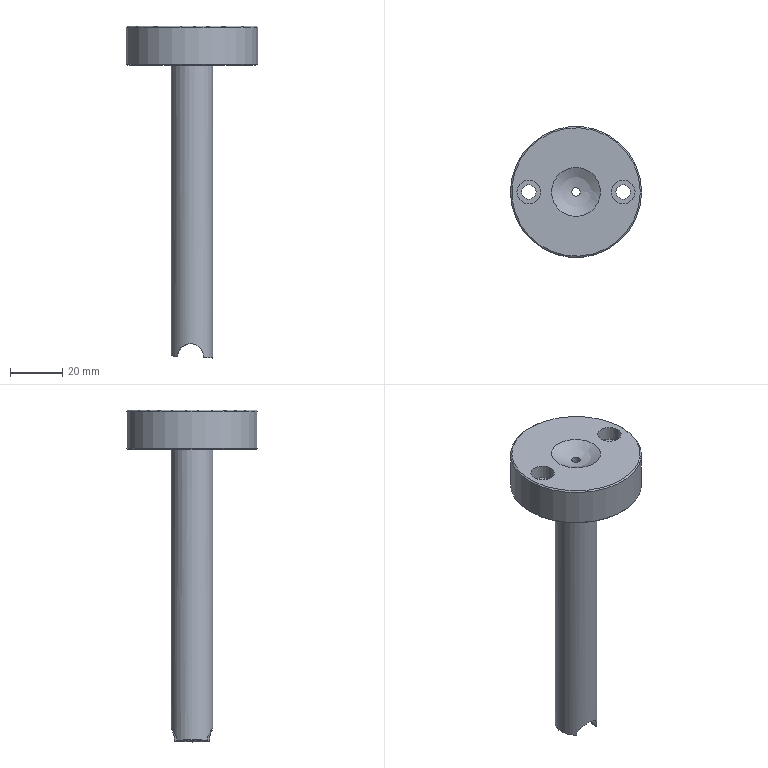Part | STEP file | solid 70 | 1 solid | 18 faces | box 50 x 50 x 126.59 mm | volume 43953 mm3 | cylinder 8 | plane 6 | cone 3 | sphere 1 | commonest cylinder face diameters 5.5 x2 9 x2 10 x2 16 x1 50 x1